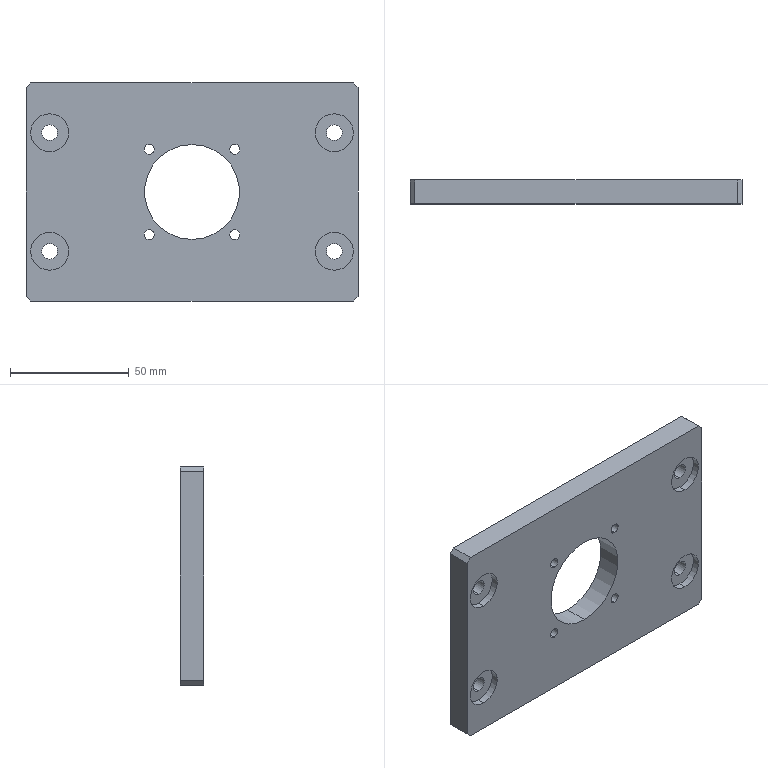Part | STEP file | PN_0037 Plate_Default | 1 solid | 52 faces | box 140 x 10 x 92 mm | volume 111742 mm3 | cylinder 34 | plane 18 | commonest cylinder face diameters 4.2 x8 6.6 x8 11 x8 16 x8 40 x2